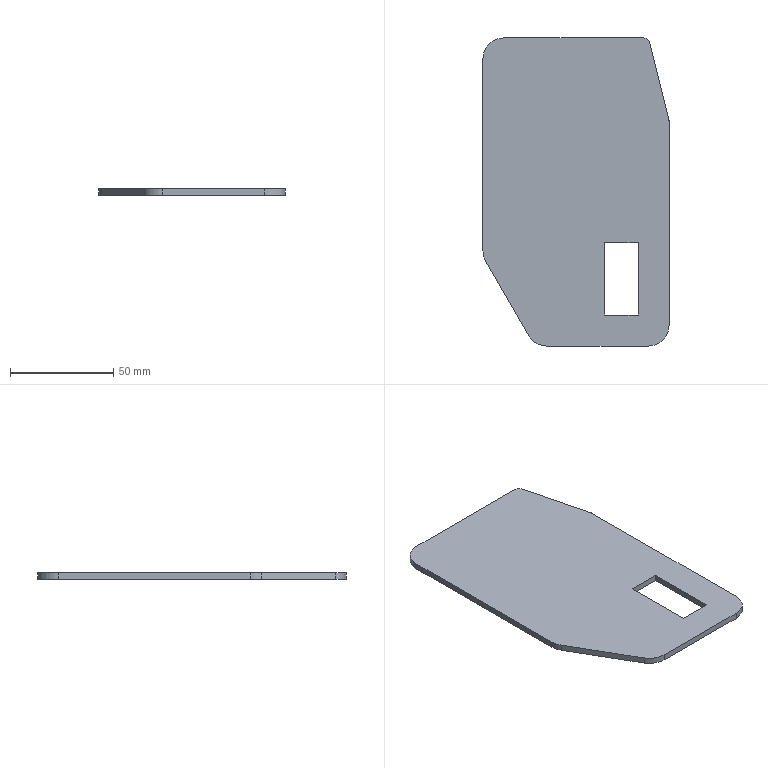Part | STEP file | Q7C1202R | 1 solid | 18 faces | box 90 x 149 x 3 mm | volume 36176 mm3 | plane 12 | cylinder 6 | commonest cylinder face diameters 20 x4 6 x2
STEP:
#1=CARTESIAN_POINT('',(0.,0.,0.));
#2=DIRECTION('',(0.,0.,1.));
#3=DIRECTION('',(1.,0.,0.));
#4=AXIS2_PLACEMENT_3D('',#1,#2,#3);
#5=CARTESIAN_POINT('',(45.,-64.5,-1.5));
#6=VERTEX_POINT('',#5);
#7=CARTESIAN_POINT('',(45.,34.131,-1.5));
#8=VERTEX_POINT('',#7);
#9=CARTESIAN_POINT('',(45.,-74.5,-1.5));
#10=DIRECTION('',(0.,1.,0.));
#11=VECTOR('',#10,1.);
#12=LINE('',#9,#11);
#13=CARTESIAN_POINT('',(45.,-74.5,1.5));
#14=DIRECTION('',(-1.,0.,0.));
#15=DIRECTION('',(0.,0.,1.));
#16=AXIS2_PLACEMENT_3D('',#13,#14,#15);
#17=PLANE('',#16);
#18=CARTESIAN_POINT('',(-3.,0.));
#19=DIRECTION('',(0.,1.));
#20=VECTOR('',#19,1.);
#21=LINE('',#18,#20);
#22=(GEOMETRIC_REPRESENTATION_CONTEXT(2)PARAMETRIC_REPRESENTATION_CONTEXT()REPRESENTATION_CONTEXT('',''));
#23=DEFINITIONAL_REPRESENTATION('',(#21),#22);
#24=PCURVE('',#17,#23);
#25=CARTESIAN_POINT('',(45.,74.5,-1.5));
#26=DIRECTION('',(0.,0.,1.));
#27=DIRECTION('',(1.,0.,0.));
#28=AXIS2_PLACEMENT_3D('',#25,#26,#27);
#29=PLANE('',#28);
#30=CARTESIAN_POINT('',(0.,-149.));
#31=DIRECTION('',(0.,1.));
#32=VECTOR('',#31,1.);
#33=LINE('',#30,#32);
#34=(GEOMETRIC_REPRESENTATION_CONTEXT(2)PARAMETRIC_REPRESENTATION_CONTEXT()REPRESENTATION_CONTEXT('',''));
#35=DEFINITIONAL_REPRESENTATION('',(#33),#34);
#36=PCURVE('',#29,#35);
#37=SURFACE_CURVE('',#12,(#24,#36),.PCURVE_S1.);
#38=EDGE_CURVE('',#6,#8,#37,.T.);
#39=ORIENTED_EDGE('',*,*,#38,.T.);
#40=CARTESIAN_POINT('',(45.,34.131,1.5));
#41=VERTEX_POINT('',#40);
#42=CARTESIAN_POINT('',(45.,34.131,1.5));
#43=DIRECTION('',(0.,0.,1.));
#44=VECTOR('',#43,1.);
#45=LINE('',#42,#44);
#46=CARTESIAN_POINT('',(0.,108.631));
#47=DIRECTION('',(1.,0.));
#48=VECTOR('',#47,1.);
#49=LINE('',#46,#48);
#50=(GEOMETRIC_REPRESENTATION_CONTEXT(2)PARAMETRIC_REPRESENTATION_CONTEXT()REPRESENTATION_CONTEXT('',''));
#51=DEFINITIONAL_REPRESENTATION('',(#49),#50);
#52=PCURVE('',#17,#51);
#53=CARTESIAN_POINT('',(42.,34.131,1.5));
#54=DIRECTION('',(0.,0.,1.));
#55=DIRECTION('',(1.,0.,0.));
#56=AXIS2_PLACEMENT_3D('',#53,#54,#55);
#57=CYLINDRICAL_SURFACE('',#56,3.);
#58=CARTESIAN_POINT('',(0.,0.));
#59=DIRECTION('',(0.,1.));
#60=VECTOR('',#59,1.);
#61=LINE('',#58,#60);
#62=(GEOMETRIC_REPRESENTATION_CONTEXT(2)PARAMETRIC_REPRESENTATION_CONTEXT()REPRESENTATION_CONTEXT('',''));
#63=DEFINITIONAL_REPRESENTATION('',(#61),#62);
#64=PCURVE('',#57,#63);
#65=SURFACE_CURVE('',#45,(#52,#64),.PCURVE_S1.);
#66=EDGE_CURVE('',#8,#41,#65,.T.);
#67=ORIENTED_EDGE('',*,*,#66,.T.);
#68=CARTESIAN_POINT('',(45.,-64.5,1.5));
#69=VERTEX_POINT('',#68);
#70=CARTESIAN_POINT('',(45.,-74.5,1.5));
#71=DIRECTION('',(0.,1.,0.));
#72=VECTOR('',#71,1.);
#73=LINE('',#70,#72);
#74=CARTESIAN_POINT('',(0.,0.));
#75=DIRECTION('',(0.,1.));
#76=VECTOR('',#75,1.);
#77=LINE('',#74,#76);
#78=(GEOMETRIC_REPRESENTATION_CONTEXT(2)PARAMETRIC_REPRESENTATION_CONTEXT()REPRESENTATION_CONTEXT('',''));
#79=DEFINITIONAL_REPRESENTATION('',(#77),#78);
#80=PCURVE('',#17,#79);
#81=CARTESIAN_POINT('',(45.,74.5,1.5));
#82=DIRECTION('',(0.,0.,1.));
#83=DIRECTION('',(1.,0.,0.));
#84=AXIS2_PLACEMENT_3D('',#81,#82,#83);
#85=PLANE('',#84);
#86=CARTESIAN_POINT('',(0.,-149.));
#87=DIRECTION('',(0.,1.));
#88=VECTOR('',#87,1.);
#89=LINE('',#86,#88);
#90=(GEOMETRIC_REPRESENTATION_CONTEXT(2)PARAMETRIC_REPRESENTATION_CONTEXT()REPRESENTATION_CONTEXT('',''));
#91=DEFINITIONAL_REPRESENTATION('',(#89),#90);
#92=PCURVE('',#85,#91);
#93=SURFACE_CURVE('',#73,(#80,#92),.PCURVE_S1.);
#94=EDGE_CURVE('',#69,#41,#93,.T.);
#95=ORIENTED_EDGE('',*,*,#94,.F.);
#96=CARTESIAN_POINT('',(45.,-64.5,1.5));
#97=DIRECTION('',(0.,0.,-1.));
#98=VECTOR('',#97,1.);
#99=LINE('',#96,#98);
#100=CARTESIAN_POINT('',(0.,10.));
#101=DIRECTION('',(-1.,0.));
#102=VECTOR('',#101,1.);
#103=LINE('',#100,#102);
#104=(GEOMETRIC_REPRESENTATION_CONTEXT(2)PARAMETRIC_REPRESENTATION_CONTEXT()REPRESENTATION_CONTEXT('',''));
#105=DEFINITIONAL_REPRESENTATION('',(#103),#104);
#106=PCURVE('',#17,#105);
#107=CARTESIAN_POINT('',(35.,-64.5,1.5));
#108=DIRECTION('',(0.,0.,-1.));
#109=DIRECTION('',(-1.,0.,0.));
#110=AXIS2_PLACEMENT_3D('',#107,#108,#109);
#111=CYLINDRICAL_SURFACE('',#110,10.);
#112=CARTESIAN_POINT('',(3.142,0.));
#113=DIRECTION('',(0.,1.));
#114=VECTOR('',#113,1.);
#115=LINE('',#112,#114);
#116=(GEOMETRIC_REPRESENTATION_CONTEXT(2)PARAMETRIC_REPRESENTATION_CONTEXT()REPRESENTATION_CONTEXT('',''));
#117=DEFINITIONAL_REPRESENTATION('',(#115),#116);
#118=PCURVE('',#111,#117);
#119=SURFACE_CURVE('',#99,(#106,#118),.PCURVE_S1.);
#120=EDGE_CURVE('',#69,#6,#119,.T.);
#121=ORIENTED_EDGE('',*,*,#120,.T.);
#122=EDGE_LOOP('',(#39,#67,#95,#121));
#123=FACE_BOUND('',#122,.T.);
#124=ADVANCED_FACE('',(#123),#17,.F.);
#125=CARTESIAN_POINT('',(32.658,74.5,1.5));
#126=VERTEX_POINT('',#125);
#127=CARTESIAN_POINT('',(-35.,74.5,1.5));
#128=VERTEX_POINT('',#127);
#129=CARTESIAN_POINT('',(45.,74.5,1.5));
#130=DIRECTION('',(-1.,0.,0.));
#131=VECTOR('',#130,1.);
#132=LINE('',#129,#131);
#133=CARTESIAN_POINT('',(45.,74.5,1.5));
#134=DIRECTION('',(0.,-1.,0.));
#135=DIRECTION('',(0.,0.,-1.));
#136=AXIS2_PLACEMENT_3D('',#133,#134,#135);
#137=PLANE('',#136);
#138=CARTESIAN_POINT('',(0.,0.));
#139=DIRECTION('',(0.,-1.));
#140=VECTOR('',#139,1.);
#141=LINE('',#138,#140);
#142=(GEOMETRIC_REPRESENTATION_CONTEXT(2)PARAMETRIC_REPRESENTATION_CONTEXT()REPRESENTATION_CONTEXT('',''));
#143=DEFINITIONAL_REPRESENTATION('',(#141),#142);
#144=PCURVE('',#137,#143);
#145=CARTESIAN_POINT('',(0.,0.));
#146=DIRECTION('',(-1.,0.));
#147=VECTOR('',#146,1.);
#148=LINE('',#145,#147);
#149=(GEOMETRIC_REPRESENTATION_CONTEXT(2)PARAMETRIC_REPRESENTATION_CONTEXT()REPRESENTATION_CONTEXT('',''));
#150=DEFINITIONAL_REPRESENTATION('',(#148),#149);
#151=PCURVE('',#85,#150);
#152=SURFACE_CURVE('',#132,(#144,#151),.PCURVE_S1.);
#153=EDGE_CURVE('',#126,#128,#152,.T.);
#154=ORIENTED_EDGE('',*,*,#153,.F.);
#155=CARTESIAN_POINT('',(32.658,74.5,-1.5));
#156=VERTEX_POINT('',#155);
#157=CARTESIAN_POINT('',(32.658,74.5,1.5));
#158=DIRECTION('',(0.,0.,-1.));
#159=VECTOR('',#158,1.);
#160=LINE('',#157,#159);
#161=CARTESIAN_POINT('',(0.,-12.342));
#162=DIRECTION('',(1.,0.));
#163=VECTOR('',#162,1.);
#164=LINE('',#161,#163);
#165=(GEOMETRIC_REPRESENTATION_CONTEXT(2)PARAMETRIC_REPRESENTATION_CONTEXT()REPRESENTATION_CONTEXT('',''));
#166=DEFINITIONAL_REPRESENTATION('',(#164),#165);
#167=PCURVE('',#137,#166);
#168=CARTESIAN_POINT('',(32.658,71.5,1.5));
#169=DIRECTION('',(0.,0.,-1.));
#170=DIRECTION('',(-1.,0.,0.));
#171=AXIS2_PLACEMENT_3D('',#168,#169,#170);
#172=CYLINDRICAL_SURFACE('',#171,3.);
#173=CARTESIAN_POINT('',(1.571,0.));
#174=DIRECTION('',(0.,1.));
#175=VECTOR('',#174,1.);
#176=LINE('',#173,#175);
#177=(GEOMETRIC_REPRESENTATION_CONTEXT(2)PARAMETRIC_REPRESENTATION_CONTEXT()REPRESENTATION_CONTEXT('',''));
#178=DEFINITIONAL_REPRESENTATION('',(#176),#177);
#179=PCURVE('',#172,#178);
#180=SURFACE_CURVE('',#160,(#167,#179),.PCURVE_S1.);
#181=EDGE_CURVE('',#126,#156,#180,.T.);
#182=ORIENTED_EDGE('',*,*,#181,.T.);
#183=CARTESIAN_POINT('',(-35.,74.5,-1.5));
#184=VERTEX_POINT('',#183);
#185=CARTESIAN_POINT('',(45.,74.5,-1.5));
#186=DIRECTION('',(-1.,0.,0.));
#187=VECTOR('',#186,1.);
#188=LINE('',#185,#187);
#189=CARTESIAN_POINT('',(3.,0.));
#190=DIRECTION('',(0.,-1.));
#191=VECTOR('',#190,1.);
#192=LINE('',#189,#191);
#193=(GEOMETRIC_REPRESENTATION_CONTEXT(2)PARAMETRIC_REPRESENTATION_CONTEXT()REPRESENTATION_CONTEXT('',''));
#194=DEFINITIONAL_REPRESENTATION('',(#192),#193);
#195=PCURVE('',#137,#194);
#196=CARTESIAN_POINT('',(0.,0.));
#197=DIRECTION('',(-1.,0.));
#198=VECTOR('',#197,1.);
#199=LINE('',#196,#198);
#200=(GEOMETRIC_REPRESENTATION_CONTEXT(2)PARAMETRIC_REPRESENTATION_CONTEXT()REPRESENTATION_CONTEXT('',''));
#201=DEFINITIONAL_REPRESENTATION('',(#199),#200);
#202=PCURVE('',#29,#201);
#203=SURFACE_CURVE('',#188,(#195,#202),.PCURVE_S1.);
#204=EDGE_CURVE('',#156,#184,#203,.T.);
#205=ORIENTED_EDGE('',*,*,#204,.T.);
#206=CARTESIAN_POINT('',(-35.,74.5,1.5));
#207=DIRECTION('',(0.,0.,1.));
#208=VECTOR('',#207,1.);
#209=LINE('',#206,#208);
#210=CARTESIAN_POINT('',(0.,-80.));
#211=DIRECTION('',(-1.,0.));
#212=VECTOR('',#211,1.);
#213=LINE('',#210,#212);
#214=(GEOMETRIC_REPRESENTATION_CONTEXT(2)PARAMETRIC_REPRESENTATION_CONTEXT()REPRESENTATION_CONTEXT('',''));
#215=DEFINITIONAL_REPRESENTATION('',(#213),#214);
#216=PCURVE('',#137,#215);
#217=CARTESIAN_POINT('',(-35.,64.5,1.5));
#218=DIRECTION('',(0.,0.,-1.));
#219=DIRECTION('',(-1.,0.,0.));
#220=AXIS2_PLACEMENT_3D('',#217,#218,#219);
#221=CYLINDRICAL_SURFACE('',#220,10.);
#222=CARTESIAN_POINT('',(1.571,0.));
#223=DIRECTION('',(0.,-1.));
#224=VECTOR('',#223,1.);
#225=LINE('',#222,#224);
#226=(GEOMETRIC_REPRESENTATION_CONTEXT(2)PARAMETRIC_REPRESENTATION_CONTEXT()REPRESENTATION_CONTEXT('',''));
#227=DEFINITIONAL_REPRESENTATION('',(#225),#226);
#228=PCURVE('',#221,#227);
#229=SURFACE_CURVE('',#209,(#216,#228),.PCURVE_S1.);
#230=EDGE_CURVE('',#184,#128,#229,.T.);
#231=ORIENTED_EDGE('',*,*,#230,.T.);
#232=EDGE_LOOP('',(#154,#182,#205,#231));
#233=FACE_BOUND('',#232,.T.);
#234=ADVANCED_FACE('',(#233),#137,.F.);
#235=CARTESIAN_POINT('',(-45.,64.5,-1.5));
#236=VERTEX_POINT('',#235);
#237=CARTESIAN_POINT('',(-45.,-28.519,-1.5));
#238=VERTEX_POINT('',#237);
#239=CARTESIAN_POINT('',(-45.,74.5,-1.5));
#240=DIRECTION('',(0.,-1.,0.));
#241=VECTOR('',#240,1.);
#242=LINE('',#239,#241);
#243=CARTESIAN_POINT('',(-45.,74.5,1.5));
#244=DIRECTION('',(1.,0.,0.));
#245=DIRECTION('',(0.,1.,0.));
#246=AXIS2_PLACEMENT_3D('',#243,#244,#245);
#247=PLANE('',#246);
#248=CARTESIAN_POINT('',(0.,-3.));
#249=DIRECTION('',(-1.,0.));
#250=VECTOR('',#249,1.);
#251=LINE('',#248,#250);
#252=(GEOMETRIC_REPRESENTATION_CONTEXT(2)PARAMETRIC_REPRESENTATION_CONTEXT()REPRESENTATION_CONTEXT('',''));
#253=DEFINITIONAL_REPRESENTATION('',(#251),#252);
#254=PCURVE('',#247,#253);
#255=CARTESIAN_POINT('',(-90.,0.));
#256=DIRECTION('',(0.,-1.));
#257=VECTOR('',#256,1.);
#258=LINE('',#255,#257);
#259=(GEOMETRIC_REPRESENTATION_CONTEXT(2)PARAMETRIC_REPRESENTATION_CONTEXT()REPRESENTATION_CONTEXT('',''));
#260=DEFINITIONAL_REPRESENTATION('',(#258),#259);
#261=PCURVE('',#29,#260);
#262=SURFACE_CURVE('',#242,(#254,#261),.PCURVE_S1.);
#263=EDGE_CURVE('',#236,#238,#262,.T.);
#264=ORIENTED_EDGE('',*,*,#263,.T.);
#265=CARTESIAN_POINT('',(-45.,-28.519,1.5));
#266=VERTEX_POINT('',#265);
#267=CARTESIAN_POINT('',(-45.,-28.519,1.5));
#268=DIRECTION('',(0.,0.,1.));
#269=VECTOR('',#268,1.);
#270=LINE('',#267,#269);
#271=CARTESIAN_POINT('',(-103.019,0.));
#272=DIRECTION('',(0.,1.));
#273=VECTOR('',#272,1.);
#274=LINE('',#271,#273);
#275=(GEOMETRIC_REPRESENTATION_CONTEXT(2)PARAMETRIC_REPRESENTATION_CONTEXT()REPRESENTATION_CONTEXT('',''));
#276=DEFINITIONAL_REPRESENTATION('',(#274),#275);
#277=PCURVE('',#247,#276);
#278=CARTESIAN_POINT('',(-35.,-28.519,1.5));
#279=DIRECTION('',(0.,0.,-1.));
#280=DIRECTION('',(-1.,0.,0.));
#281=AXIS2_PLACEMENT_3D('',#278,#279,#280);
#282=CYLINDRICAL_SURFACE('',#281,10.);
#283=CARTESIAN_POINT('',(6.283,0.));
#284=DIRECTION('',(0.,-1.));
#285=VECTOR('',#284,1.);
#286=LINE('',#283,#285);
#287=(GEOMETRIC_REPRESENTATION_CONTEXT(2)PARAMETRIC_REPRESENTATION_CONTEXT()REPRESENTATION_CONTEXT('',''));
#288=DEFINITIONAL_REPRESENTATION('',(#286),#287);
#289=PCURVE('',#282,#288);
#290=SURFACE_CURVE('',#270,(#277,#289),.PCURVE_S1.);
#291=EDGE_CURVE('',#238,#266,#290,.T.);
#292=ORIENTED_EDGE('',*,*,#291,.T.);
#293=CARTESIAN_POINT('',(-45.,64.5,1.5));
#294=VERTEX_POINT('',#293);
#295=CARTESIAN_POINT('',(-45.,74.5,1.5));
#296=DIRECTION('',(0.,-1.,0.));
#297=VECTOR('',#296,1.);
#298=LINE('',#295,#297);
#299=CARTESIAN_POINT('',(0.,0.));
#300=DIRECTION('',(-1.,0.));
#301=VECTOR('',#300,1.);
#302=LINE('',#299,#301);
#303=(GEOMETRIC_REPRESENTATION_CONTEXT(2)PARAMETRIC_REPRESENTATION_CONTEXT()REPRESENTATION_CONTEXT('',''));
#304=DEFINITIONAL_REPRESENTATION('',(#302),#303);
#305=PCURVE('',#247,#304);
#306=CARTESIAN_POINT('',(-90.,0.));
#307=DIRECTION('',(0.,-1.));
#308=VECTOR('',#307,1.);
#309=LINE('',#306,#308);
#310=(GEOMETRIC_REPRESENTATION_CONTEXT(2)PARAMETRIC_REPRESENTATION_CONTEXT()REPRESENTATION_CONTEXT('',''));
#311=DEFINITIONAL_REPRESENTATION('',(#309),#310);
#312=PCURVE('',#85,#311);
#313=SURFACE_CURVE('',#298,(#305,#312),.PCURVE_S1.);
#314=EDGE_CURVE('',#294,#266,#313,.T.);
#315=ORIENTED_EDGE('',*,*,#314,.F.);
#316=CARTESIAN_POINT('',(-45.,64.5,1.5));
#317=DIRECTION('',(0.,0.,-1.));
#318=VECTOR('',#317,1.);
#319=LINE('',#316,#318);
#320=CARTESIAN_POINT('',(-10.,0.));
#321=DIRECTION('',(0.,-1.));
#322=VECTOR('',#321,1.);
#323=LINE('',#320,#322);
#324=(GEOMETRIC_REPRESENTATION_CONTEXT(2)PARAMETRIC_REPRESENTATION_CONTEXT()REPRESENTATION_CONTEXT('',''));
#325=DEFINITIONAL_REPRESENTATION('',(#323),#324);
#326=PCURVE('',#247,#325);
#327=CARTESIAN_POINT('',(0.,0.));
#328=DIRECTION('',(0.,1.));
#329=VECTOR('',#328,1.);
#330=LINE('',#327,#329);
#331=(GEOMETRIC_REPRESENTATION_CONTEXT(2)PARAMETRIC_REPRESENTATION_CONTEXT()REPRESENTATION_CONTEXT('',''));
#332=DEFINITIONAL_REPRESENTATION('',(#330),#331);
#333=PCURVE('',#221,#332);
#334=SURFACE_CURVE('',#319,(#326,#333),.PCURVE_S1.);
#335=EDGE_CURVE('',#294,#236,#334,.T.);
#336=ORIENTED_EDGE('',*,*,#335,.T.);
#337=EDGE_LOOP('',(#264,#292,#315,#336));
#338=FACE_BOUND('',#337,.T.);
#339=ADVANCED_FACE('',(#338),#247,.F.);
#340=CARTESIAN_POINT('',(-43.66,-33.519,1.5));
#341=VERTEX_POINT('',#340);
#342=CARTESIAN_POINT('',(-22.887,-69.5,1.5));
#343=VERTEX_POINT('',#342);
#344=CARTESIAN_POINT('',(-45.,-31.199,1.5));
#345=DIRECTION('',(0.5,-0.866,0.));
#346=VECTOR('',#345,1.);
#347=LINE('',#344,#346);
#348=CARTESIAN_POINT('',(-45.,-31.199,1.5));
#349=DIRECTION('',(0.866,0.5,0.));
#350=DIRECTION('',(-0.5,0.866,0.));
#351=AXIS2_PLACEMENT_3D('',#348,#349,#350);
#352=PLANE('',#351);
#353=CARTESIAN_POINT('',(0.,0.));
#354=DIRECTION('',(-1.,0.));
#355=VECTOR('',#354,1.);
#356=LINE('',#353,#355);
#357=(GEOMETRIC_REPRESENTATION_CONTEXT(2)PARAMETRIC_REPRESENTATION_CONTEXT()REPRESENTATION_CONTEXT('',''));
#358=DEFINITIONAL_REPRESENTATION('',(#356),#357);
#359=PCURVE('',#352,#358);
#360=CARTESIAN_POINT('',(-90.,-105.699));
#361=DIRECTION('',(0.5,-0.866));
#362=VECTOR('',#361,1.);
#363=LINE('',#360,#362);
#364=(GEOMETRIC_REPRESENTATION_CONTEXT(2)PARAMETRIC_REPRESENTATION_CONTEXT()REPRESENTATION_CONTEXT('',''));
#365=DEFINITIONAL_REPRESENTATION('',(#363),#364);
#366=PCURVE('',#85,#365);
#367=SURFACE_CURVE('',#347,(#359,#366),.PCURVE_S1.);
#368=EDGE_CURVE('',#341,#343,#367,.T.);
#369=ORIENTED_EDGE('',*,*,#368,.F.);
#370=CARTESIAN_POINT('',(-43.66,-33.519,-1.5));
#371=VERTEX_POINT('',#370);
#372=CARTESIAN_POINT('',(-43.66,-33.519,1.5));
#373=DIRECTION('',(0.,0.,-1.));
#374=VECTOR('',#373,1.);
#375=LINE('',#372,#374);
#376=CARTESIAN_POINT('',(-2.679,0.));
#377=DIRECTION('',(0.,-1.));
#378=VECTOR('',#377,1.);
#379=LINE('',#376,#378);
#380=(GEOMETRIC_REPRESENTATION_CONTEXT(2)PARAMETRIC_REPRESENTATION_CONTEXT()REPRESENTATION_CONTEXT('',''));
#381=DEFINITIONAL_REPRESENTATION('',(#379),#380);
#382=PCURVE('',#352,#381);
#383=CARTESIAN_POINT('',(5.76,0.));
#384=DIRECTION('',(0.,1.));
#385=VECTOR('',#384,1.);
#386=LINE('',#383,#385);
#387=(GEOMETRIC_REPRESENTATION_CONTEXT(2)PARAMETRIC_REPRESENTATION_CONTEXT()REPRESENTATION_CONTEXT('',''));
#388=DEFINITIONAL_REPRESENTATION('',(#386),#387);
#389=PCURVE('',#282,#388);
#390=SURFACE_CURVE('',#375,(#382,#389),.PCURVE_S1.);
#391=EDGE_CURVE('',#341,#371,#390,.T.);
#392=ORIENTED_EDGE('',*,*,#391,.T.);
#393=CARTESIAN_POINT('',(-22.887,-69.5,-1.5));
#394=VERTEX_POINT('',#393);
#395=CARTESIAN_POINT('',(-45.,-31.199,-1.5));
#396=DIRECTION('',(0.5,-0.866,0.));
#397=VECTOR('',#396,1.);
#398=LINE('',#395,#397);
#399=CARTESIAN_POINT('',(0.,-3.));
#400=DIRECTION('',(-1.,0.));
#401=VECTOR('',#400,1.);
#402=LINE('',#399,#401);
#403=(GEOMETRIC_REPRESENTATION_CONTEXT(2)PARAMETRIC_REPRESENTATION_CONTEXT()REPRESENTATION_CONTEXT('',''));
#404=DEFINITIONAL_REPRESENTATION('',(#402),#403);
#405=PCURVE('',#352,#404);
#406=CARTESIAN_POINT('',(-90.,-105.699));
#407=DIRECTION('',(0.5,-0.866));
#408=VECTOR('',#407,1.);
#409=LINE('',#406,#408);
#410=(GEOMETRIC_REPRESENTATION_CONTEXT(2)PARAMETRIC_REPRESENTATION_CONTEXT()REPRESENTATION_CONTEXT('',''));
#411=DEFINITIONAL_REPRESENTATION('',(#409),#410);
#412=PCURVE('',#29,#411);
#413=SURFACE_CURVE('',#398,(#405,#412),.PCURVE_S1.);
#414=EDGE_CURVE('',#371,#394,#413,.T.);
#415=ORIENTED_EDGE('',*,*,#414,.T.);
#416=CARTESIAN_POINT('',(-22.887,-69.5,1.5));
#417=DIRECTION('',(0.,0.,1.));
#418=VECTOR('',#417,1.);
#419=LINE('',#416,#418);
#420=CARTESIAN_POINT('',(-44.226,0.));
#421=DIRECTION('',(0.,1.));
#422=VECTOR('',#421,1.);
#423=LINE('',#420,#422);
#424=(GEOMETRIC_REPRESENTATION_CONTEXT(2)PARAMETRIC_REPRESENTATION_CONTEXT()REPRESENTATION_CONTEXT('',''));
#425=DEFINITIONAL_REPRESENTATION('',(#423),#424);
#426=PCURVE('',#352,#425);
#427=CARTESIAN_POINT('',(-14.226,-64.5,1.5));
#428=DIRECTION('',(0.,0.,-1.));
#429=DIRECTION('',(-1.,0.,0.));
#430=AXIS2_PLACEMENT_3D('',#427,#428,#429);
#431=CYLINDRICAL_SURFACE('',#430,10.);
#432=CARTESIAN_POINT('',(5.76,0.));
#433=DIRECTION('',(0.,-1.));
#434=VECTOR('',#433,1.);
#435=LINE('',#432,#434);
#436=(GEOMETRIC_REPRESENTATION_CONTEXT(2)PARAMETRIC_REPRESENTATION_CONTEXT()REPRESENTATION_CONTEXT('',''));
#437=DEFINITIONAL_REPRESENTATION('',(#435),#436);
#438=PCURVE('',#431,#437);
#439=SURFACE_CURVE('',#419,(#426,#438),.PCURVE_S1.);
#440=EDGE_CURVE('',#394,#343,#439,.T.);
#441=ORIENTED_EDGE('',*,*,#440,.T.);
#442=EDGE_LOOP('',(#369,#392,#415,#441));
#443=FACE_BOUND('',#442,.T.);
#444=ADVANCED_FACE('',(#443),#352,.F.);
#445=CARTESIAN_POINT('',(-14.226,-74.5,1.5));
#446=VERTEX_POINT('',#445);
#447=CARTESIAN_POINT('',(35.,-74.5,1.5));
#448=VERTEX_POINT('',#447);
#449=CARTESIAN_POINT('',(-20.,-74.5,1.5));
#450=DIRECTION('',(1.,0.,0.));
#451=VECTOR('',#450,1.);
#452=LINE('',#449,#451);
#453=CARTESIAN_POINT('',(-20.,-74.5,1.5));
#454=DIRECTION('',(0.,1.,0.));
#455=DIRECTION('',(0.,0.,1.));
#456=AXIS2_PLACEMENT_3D('',#453,#454,#455);
#457=PLANE('',#456);
#458=CARTESIAN_POINT('',(0.,0.));
#459=DIRECTION('',(0.,1.));
#460=VECTOR('',#459,1.);
#461=LINE('',#458,#460);
#462=(GEOMETRIC_REPRESENTATION_CONTEXT(2)PARAMETRIC_REPRESENTATION_CONTEXT()REPRESENTATION_CONTEXT('',''));
#463=DEFINITIONAL_REPRESENTATION('',(#461),#462);
#464=PCURVE('',#457,#463);
#465=CARTESIAN_POINT('',(-65.,-149.));
#466=DIRECTION('',(1.,0.));
#467=VECTOR('',#466,1.);
#468=LINE('',#465,#467);
#469=(GEOMETRIC_REPRESENTATION_CONTEXT(2)PARAMETRIC_REPRESENTATION_CONTEXT()REPRESENTATION_CONTEXT('',''));
#470=DEFINITIONAL_REPRESENTATION('',(#468),#469);
#471=PCURVE('',#85,#470);
#472=SURFACE_CURVE('',#452,(#464,#471),.PCURVE_S1.);
#473=EDGE_CURVE('',#446,#448,#472,.T.);
#474=ORIENTED_EDGE('',*,*,#473,.F.);
#475=CARTESIAN_POINT('',(-14.226,-74.5,-1.5));
#476=VERTEX_POINT('',#475);
#477=CARTESIAN_POINT('',(-14.226,-74.5,1.5));
#478=DIRECTION('',(0.,0.,-1.));
#479=VECTOR('',#478,1.);
#480=LINE('',#477,#479);
#481=CARTESIAN_POINT('',(0.,5.774));
#482=DIRECTION('',(-1.,0.));
#483=VECTOR('',#482,1.);
#484=LINE('',#481,#483);
#485=(GEOMETRIC_REPRESENTATION_CONTEXT(2)PARAMETRIC_REPRESENTATION_CONTEXT()REPRESENTATION_CONTEXT('',''));
#486=DEFINITIONAL_REPRESENTATION('',(#484),#485);
#487=PCURVE('',#457,#486);
#488=CARTESIAN_POINT('',(4.712,0.));
#489=DIRECTION('',(0.,1.));
#490=VECTOR('',#489,1.);
#491=LINE('',#488,#490);
#492=(GEOMETRIC_REPRESENTATION_CONTEXT(2)PARAMETRIC_REPRESENTATION_CONTEXT()REPRESENTATION_CONTEXT('',''));
#493=DEFINITIONAL_REPRESENTATION('',(#491),#492);
#494=PCURVE('',#431,#493);
#495=SURFACE_CURVE('',#480,(#487,#494),.PCURVE_S1.);
#496=EDGE_CURVE('',#446,#476,#495,.T.);
#497=ORIENTED_EDGE('',*,*,#496,.T.);
#498=CARTESIAN_POINT('',(35.,-74.5,-1.5));
#499=VERTEX_POINT('',#498);
#500=CARTESIAN_POINT('',(-20.,-74.5,-1.5));
#501=DIRECTION('',(1.,0.,0.));
#502=VECTOR('',#501,1.);
#503=LINE('',#500,#502);
#504=CARTESIAN_POINT('',(-3.,0.));
#505=DIRECTION('',(0.,1.));
#506=VECTOR('',#505,1.);
#507=LINE('',#504,#506);
#508=(GEOMETRIC_REPRESENTATION_CONTEXT(2)PARAMETRIC_REPRESENTATION_CONTEXT()REPRESENTATION_CONTEXT('',''));
#509=DEFINITIONAL_REPRESENTATION('',(#507),#508);
#510=PCURVE('',#457,#509);
#511=CARTESIAN_POINT('',(-65.,-149.));
#512=DIRECTION('',(1.,0.));
#513=VECTOR('',#512,1.);
#514=LINE('',#511,#513);
#515=(GEOMETRIC_REPRESENTATION_CONTEXT(2)PARAMETRIC_REPRESENTATION_CONTEXT()REPRESENTATION_CONTEXT('',''));
#516=DEFINITIONAL_REPRESENTATION('',(#514),#515);
#517=PCURVE('',#29,#516);
#518=SURFACE_CURVE('',#503,(#510,#517),.PCURVE_S1.);
#519=EDGE_CURVE('',#476,#499,#518,.T.);
#520=ORIENTED_EDGE('',*,*,#519,.T.);
#521=CARTESIAN_POINT('',(35.,-74.5,1.5));
#522=DIRECTION('',(0.,0.,1.));
#523=VECTOR('',#522,1.);
#524=LINE('',#521,#523);
#525=CARTESIAN_POINT('',(0.,55.));
#526=DIRECTION('',(1.,0.));
#527=VECTOR('',#526,1.);
#528=LINE('',#525,#527);
#529=(GEOMETRIC_REPRESENTATION_CONTEXT(2)PARAMETRIC_REPRESENTATION_CONTEXT()REPRESENTATION_CONTEXT('',''));
#530=DEFINITIONAL_REPRESENTATION('',(#528),#529);
#531=PCURVE('',#457,#530);
#532=CARTESIAN_POINT('',(4.712,0.));
#533=DIRECTION('',(0.,-1.));
#534=VECTOR('',#533,1.);
#535=LINE('',#532,#534);
#536=(GEOMETRIC_REPRESENTATION_CONTEXT(2)PARAMETRIC_REPRESENTATION_CONTEXT()REPRESENTATION_CONTEXT('',''));
#537=DEFINITIONAL_REPRESENTATION('',(#535),#536);
#538=PCURVE('',#111,#537);
#539=SURFACE_CURVE('',#524,(#531,#538),.PCURVE_S1.);
#540=EDGE_CURVE('',#499,#448,#539,.T.);
#541=ORIENTED_EDGE('',*,*,#540,.T.);
#542=EDGE_LOOP('',(#474,#497,#520,#541));
#543=FACE_BOUND('',#542,.T.);
#544=ADVANCED_FACE('',(#543),#457,.F.);
#545=ORIENTED_EDGE('',*,*,#94,.T.);
#546=CARTESIAN_POINT('',(44.91,34.858,1.5));
#547=VERTEX_POINT('',#546);
#548=CARTESIAN_POINT('',(42.,34.131,1.5));
#549=DIRECTION('',(0.,0.,1.));
#550=DIRECTION('',(1.,0.,0.));
#551=AXIS2_PLACEMENT_3D('',#548,#549,#550);
#552=CIRCLE('',#551,3.);
#553=CARTESIAN_POINT('',(-3.,-40.369));
#554=DIRECTION('',(1.,0.));
#555=AXIS2_PLACEMENT_2D('',#553,#554);
#556=CIRCLE('',#555,3.);
#557=(GEOMETRIC_REPRESENTATION_CONTEXT(2)PARAMETRIC_REPRESENTATION_CONTEXT()REPRESENTATION_CONTEXT('',''));
#558=DEFINITIONAL_REPRESENTATION('',(#556),#557);
#559=PCURVE('',#85,#558);
#560=CARTESIAN_POINT('',(0.,0.));
#561=DIRECTION('',(1.,0.));
#562=VECTOR('',#561,1.);
#563=LINE('',#560,#562);
#564=(GEOMETRIC_REPRESENTATION_CONTEXT(2)PARAMETRIC_REPRESENTATION_CONTEXT()REPRESENTATION_CONTEXT('',''));
#565=DEFINITIONAL_REPRESENTATION('',(#563),#564);
#566=PCURVE('',#57,#565);
#567=SURFACE_CURVE('',#552,(#559,#566),.PCURVE_S1.);
#568=EDGE_CURVE('',#41,#547,#567,.T.);
#569=ORIENTED_EDGE('',*,*,#568,.T.);
#570=CARTESIAN_POINT('',(35.568,72.228,1.5));
#571=VERTEX_POINT('',#570);
#572=CARTESIAN_POINT('',(35.,74.5,1.5));
#573=DIRECTION('',(0.2425,-0.9701,0.));
#574=VECTOR('',#573,1.);
#575=LINE('',#572,#574);
#576=CARTESIAN_POINT('',(-10.,0.));
#577=DIRECTION('',(0.2425,-0.9701));
#578=VECTOR('',#577,1.);
#579=LINE('',#576,#578);
#580=(GEOMETRIC_REPRESENTATION_CONTEXT(2)PARAMETRIC_REPRESENTATION_CONTEXT()REPRESENTATION_CONTEXT('',''));
#581=DEFINITIONAL_REPRESENTATION('',(#579),#580);
#582=PCURVE('',#85,#581);
#583=CARTESIAN_POINT('',(35.,74.5,-8.5));
#584=DIRECTION('',(-0.9701,-0.2425,0.));
#585=DIRECTION('',(0.2425,-0.9701,0.));
#586=AXIS2_PLACEMENT_3D('',#583,#584,#585);
#587=PLANE('',#586);
#588=CARTESIAN_POINT('',(0.,10.));
#589=DIRECTION('',(1.,0.));
#590=VECTOR('',#589,1.);
#591=LINE('',#588,#590);
#592=(GEOMETRIC_REPRESENTATION_CONTEXT(2)PARAMETRIC_REPRESENTATION_CONTEXT()REPRESENTATION_CONTEXT('',''));
#593=DEFINITIONAL_REPRESENTATION('',(#591),#592);
#594=PCURVE('',#587,#593);
#595=SURFACE_CURVE('',#575,(#582,#594),.PCURVE_S1.);
#596=EDGE_CURVE('',#571,#547,#595,.T.);
#597=ORIENTED_EDGE('',*,*,#596,.F.);
#598=CARTESIAN_POINT('',(32.658,71.5,1.5));
#599=DIRECTION('',(0.,0.,1.));
#600=DIRECTION('',(1.,0.,0.));
#601=AXIS2_PLACEMENT_3D('',#598,#599,#600);
#602=CIRCLE('',#601,3.);
#603=CARTESIAN_POINT('',(-12.342,-3.));
#604=DIRECTION('',(1.,0.));
#605=AXIS2_PLACEMENT_2D('',#603,#604);
#606=CIRCLE('',#605,3.);
#607=(GEOMETRIC_REPRESENTATION_CONTEXT(2)PARAMETRIC_REPRESENTATION_CONTEXT()REPRESENTATION_CONTEXT('',''));
#608=DEFINITIONAL_REPRESENTATION('',(#606),#607);
#609=PCURVE('',#85,#608);
#610=CARTESIAN_POINT('',(3.142,0.));
#611=DIRECTION('',(-1.,0.));
#612=VECTOR('',#611,1.);
#613=LINE('',#610,#612);
#614=(GEOMETRIC_REPRESENTATION_CONTEXT(2)PARAMETRIC_REPRESENTATION_CONTEXT()REPRESENTATION_CONTEXT('',''));
#615=DEFINITIONAL_REPRESENTATION('',(#613),#614);
#616=PCURVE('',#172,#615);
#617=SURFACE_CURVE('',#602,(#609,#616),.PCURVE_S1.);
#618=EDGE_CURVE('',#571,#126,#617,.T.);
#619=ORIENTED_EDGE('',*,*,#618,.T.);
#620=ORIENTED_EDGE('',*,*,#153,.T.);
#621=CARTESIAN_POINT('',(-35.,64.5,1.5));
#622=DIRECTION('',(0.,0.,1.));
#623=DIRECTION('',(1.,0.,0.));
#624=AXIS2_PLACEMENT_3D('',#621,#622,#623);
#625=CIRCLE('',#624,10.);
#626=CARTESIAN_POINT('',(-80.,-10.));
#627=DIRECTION('',(1.,0.));
#628=AXIS2_PLACEMENT_2D('',#626,#627);
#629=CIRCLE('',#628,10.);
#630=(GEOMETRIC_REPRESENTATION_CONTEXT(2)PARAMETRIC_REPRESENTATION_CONTEXT()REPRESENTATION_CONTEXT('',''));
#631=DEFINITIONAL_REPRESENTATION('',(#629),#630);
#632=PCURVE('',#85,#631);
#633=CARTESIAN_POINT('',(3.142,0.));
#634=DIRECTION('',(-1.,0.));
#635=VECTOR('',#634,1.);
#636=LINE('',#633,#635);
#637=(GEOMETRIC_REPRESENTATION_CONTEXT(2)PARAMETRIC_REPRESENTATION_CONTEXT()REPRESENTATION_CONTEXT('',''));
#638=DEFINITIONAL_REPRESENTATION('',(#636),#637);
#639=PCURVE('',#221,#638);
#640=SURFACE_CURVE('',#625,(#632,#639),.PCURVE_S1.);
#641=EDGE_CURVE('',#128,#294,#640,.T.);
#642=ORIENTED_EDGE('',*,*,#641,.T.);
#643=ORIENTED_EDGE('',*,*,#314,.T.);
#644=CARTESIAN_POINT('',(-35.,-28.519,1.5));
#645=DIRECTION('',(0.,0.,1.));
#646=DIRECTION('',(1.,0.,0.));
#647=AXIS2_PLACEMENT_3D('',#644,#645,#646);
#648=CIRCLE('',#647,10.);
#649=CARTESIAN_POINT('',(-80.,-103.019));
#650=DIRECTION('',(1.,0.));
#651=AXIS2_PLACEMENT_2D('',#649,#650);
#652=CIRCLE('',#651,10.);
#653=(GEOMETRIC_REPRESENTATION_CONTEXT(2)PARAMETRIC_REPRESENTATION_CONTEXT()REPRESENTATION_CONTEXT('',''));
#654=DEFINITIONAL_REPRESENTATION('',(#652),#653);
#655=PCURVE('',#85,#654);
#656=CARTESIAN_POINT('',(9.425,0.));
#657=DIRECTION('',(-1.,0.));
#658=VECTOR('',#657,1.);
#659=LINE('',#656,#658);
#660=(GEOMETRIC_REPRESENTATION_CONTEXT(2)PARAMETRIC_REPRESENTATION_CONTEXT()REPRESENTATION_CONTEXT('',''));
#661=DEFINITIONAL_REPRESENTATION('',(#659),#660);
#662=PCURVE('',#282,#661);
#663=SURFACE_CURVE('',#648,(#655,#662),.PCURVE_S1.);
#664=EDGE_CURVE('',#266,#341,#663,.T.);
#665=ORIENTED_EDGE('',*,*,#664,.T.);
#666=ORIENTED_EDGE('',*,*,#368,.T.);
#667=CARTESIAN_POINT('',(-14.226,-64.5,1.5));
#668=DIRECTION('',(0.,0.,1.));
#669=DIRECTION('',(1.,0.,0.));
#670=AXIS2_PLACEMENT_3D('',#667,#668,#669);
#671=CIRCLE('',#670,10.);
#672=CARTESIAN_POINT('',(-59.226,-139.));
#673=DIRECTION('',(1.,0.));
#674=AXIS2_PLACEMENT_2D('',#672,#673);
#675=CIRCLE('',#674,10.);
#676=(GEOMETRIC_REPRESENTATION_CONTEXT(2)PARAMETRIC_REPRESENTATION_CONTEXT()REPRESENTATION_CONTEXT('',''));
#677=DEFINITIONAL_REPRESENTATION('',(#675),#676);
#678=PCURVE('',#85,#677);
#679=CARTESIAN_POINT('',(9.425,0.));
#680=DIRECTION('',(-1.,0.));
#681=VECTOR('',#680,1.);
#682=LINE('',#679,#681);
#683=(GEOMETRIC_REPRESENTATION_CONTEXT(2)PARAMETRIC_REPRESENTATION_CONTEXT()REPRESENTATION_CONTEXT('',''));
#684=DEFINITIONAL_REPRESENTATION('',(#682),#683);
#685=PCURVE('',#431,#684);
#686=SURFACE_CURVE('',#671,(#678,#685),.PCURVE_S1.);
#687=EDGE_CURVE('',#343,#446,#686,.T.);
#688=ORIENTED_EDGE('',*,*,#687,.T.);
#689=ORIENTED_EDGE('',*,*,#473,.T.);
#690=CARTESIAN_POINT('',(35.,-64.5,1.5));
#691=DIRECTION('',(0.,0.,1.));
#692=DIRECTION('',(1.,0.,0.));
#693=AXIS2_PLACEMENT_3D('',#690,#691,#692);
#694=CIRCLE('',#693,10.);
#695=CARTESIAN_POINT('',(-10.,-139.));
#696=DIRECTION('',(1.,0.));
#697=AXIS2_PLACEMENT_2D('',#695,#696);
#698=CIRCLE('',#697,10.);
#699=(GEOMETRIC_REPRESENTATION_CONTEXT(2)PARAMETRIC_REPRESENTATION_CONTEXT()REPRESENTATION_CONTEXT('',''));
#700=DEFINITIONAL_REPRESENTATION('',(#698),#699);
#701=PCURVE('',#85,#700);
#702=CARTESIAN_POINT('',(9.425,0.));
#703=DIRECTION('',(-1.,0.));
#704=VECTOR('',#703,1.);
#705=LINE('',#702,#704);
#706=(GEOMETRIC_REPRESENTATION_CONTEXT(2)PARAMETRIC_REPRESENTATION_CONTEXT()REPRESENTATION_CONTEXT('',''));
#707=DEFINITIONAL_REPRESENTATION('',(#705),#706);
#708=PCURVE('',#111,#707);
#709=SURFACE_CURVE('',#694,(#701,#708),.PCURVE_S1.);
#710=EDGE_CURVE('',#448,#69,#709,.T.);
#711=ORIENTED_EDGE('',*,*,#710,.T.);
#712=EDGE_LOOP('',(#545,#569,#597,#619,#620,#642,#643,#665,#666,#688,#689,#711));
#713=FACE_BOUND('',#712,.T.);
#714=CARTESIAN_POINT('',(14.,-24.5,1.5));
#715=VERTEX_POINT('',#714);
#716=CARTESIAN_POINT('',(14.,-59.5,1.5));
#717=VERTEX_POINT('',#716);
#718=CARTESIAN_POINT('',(14.,-24.5,1.5));
#719=DIRECTION('',(0.,-1.,0.));
#720=VECTOR('',#719,1.);
#721=LINE('',#718,#720);
#722=CARTESIAN_POINT('',(-31.,-99.));
#723=DIRECTION('',(0.,-1.));
#724=VECTOR('',#723,1.);
#725=LINE('',#722,#724);
#726=(GEOMETRIC_REPRESENTATION_CONTEXT(2)PARAMETRIC_REPRESENTATION_CONTEXT()REPRESENTATION_CONTEXT('',''));
#727=DEFINITIONAL_REPRESENTATION('',(#725),#726);
#728=PCURVE('',#85,#727);
#729=CARTESIAN_POINT('',(14.,-24.5,-1.5));
#730=DIRECTION('',(-1.,0.,0.));
#731=DIRECTION('',(0.,-1.,0.));
#732=AXIS2_PLACEMENT_3D('',#729,#730,#731);
#733=PLANE('',#732);
#734=CARTESIAN_POINT('',(0.,3.));
#735=DIRECTION('',(1.,0.));
#736=VECTOR('',#735,1.);
#737=LINE('',#734,#736);
#738=(GEOMETRIC_REPRESENTATION_CONTEXT(2)PARAMETRIC_REPRESENTATION_CONTEXT()REPRESENTATION_CONTEXT('',''));
#739=DEFINITIONAL_REPRESENTATION('',(#737),#738);
#740=PCURVE('',#733,#739);
#741=SURFACE_CURVE('',#721,(#728,#740),.PCURVE_S1.);
#742=EDGE_CURVE('',#715,#717,#741,.T.);
#743=ORIENTED_EDGE('',*,*,#742,.F.);
#744=CARTESIAN_POINT('',(30.,-24.5,1.5));
#745=VERTEX_POINT('',#744);
#746=CARTESIAN_POINT('',(14.,-24.5,1.5));
#747=DIRECTION('',(-1.,0.,0.));
#748=VECTOR('',#747,1.);
#749=LINE('',#746,#748);
#750=CARTESIAN_POINT('',(-31.,-99.));
#751=DIRECTION('',(-1.,0.));
#752=VECTOR('',#751,1.);
#753=LINE('',#750,#752);
#754=(GEOMETRIC_REPRESENTATION_CONTEXT(2)PARAMETRIC_REPRESENTATION_CONTEXT()REPRESENTATION_CONTEXT('',''));
#755=DEFINITIONAL_REPRESENTATION('',(#753),#754);
#756=PCURVE('',#85,#755);
#757=CARTESIAN_POINT('',(14.,-24.5,-1.5));
#758=DIRECTION('',(0.,1.,0.));
#759=DIRECTION('',(0.,0.,1.));
#760=AXIS2_PLACEMENT_3D('',#757,#758,#759);
#761=PLANE('',#760);
#762=CARTESIAN_POINT('',(3.,0.));
#763=DIRECTION('',(0.,-1.));
#764=VECTOR('',#763,1.);
#765=LINE('',#762,#764);
#766=(GEOMETRIC_REPRESENTATION_CONTEXT(2)PARAMETRIC_REPRESENTATION_CONTEXT()REPRESENTATION_CONTEXT('',''));
#767=DEFINITIONAL_REPRESENTATION('',(#765),#766);
#768=PCURVE('',#761,#767);
#769=SURFACE_CURVE('',#749,(#756,#768),.PCURVE_S1.);
#770=EDGE_CURVE('',#745,#715,#769,.T.);
#771=ORIENTED_EDGE('',*,*,#770,.F.);
#772=CARTESIAN_POINT('',(30.,-59.5,1.5));
#773=VERTEX_POINT('',#772);
#774=CARTESIAN_POINT('',(30.,-24.5,1.5));
#775=DIRECTION('',(0.,1.,0.));
#776=VECTOR('',#775,1.);
#777=LINE('',#774,#776);
#778=CARTESIAN_POINT('',(-15.,-99.));
#779=DIRECTION('',(0.,1.));
#780=VECTOR('',#779,1.);
#781=LINE('',#778,#780);
#782=(GEOMETRIC_REPRESENTATION_CONTEXT(2)PARAMETRIC_REPRESENTATION_CONTEXT()REPRESENTATION_CONTEXT('',''));
#783=DEFINITIONAL_REPRESENTATION('',(#781),#782);
#784=PCURVE('',#85,#783);
#785=CARTESIAN_POINT('',(30.,-24.5,-1.5));
#786=DIRECTION('',(1.,0.,0.));
#787=DIRECTION('',(0.,1.,0.));
#788=AXIS2_PLACEMENT_3D('',#785,#786,#787);
#789=PLANE('',#788);
#790=CARTESIAN_POINT('',(0.,3.));
#791=DIRECTION('',(1.,0.));
#792=VECTOR('',#791,1.);
#793=LINE('',#790,#792);
#794=(GEOMETRIC_REPRESENTATION_CONTEXT(2)PARAMETRIC_REPRESENTATION_CONTEXT()REPRESENTATION_CONTEXT('',''));
#795=DEFINITIONAL_REPRESENTATION('',(#793),#794);
#796=PCURVE('',#789,#795);
#797=SURFACE_CURVE('',#777,(#784,#796),.PCURVE_S1.);
#798=EDGE_CURVE('',#773,#745,#797,.T.);
#799=ORIENTED_EDGE('',*,*,#798,.F.);
#800=CARTESIAN_POINT('',(14.,-59.5,1.5));
#801=DIRECTION('',(1.,0.,0.));
#802=VECTOR('',#801,1.);
#803=LINE('',#800,#802);
#804=CARTESIAN_POINT('',(-31.,-134.));
#805=DIRECTION('',(1.,0.));
#806=VECTOR('',#805,1.);
#807=LINE('',#804,#806);
#808=(GEOMETRIC_REPRESENTATION_CONTEXT(2)PARAMETRIC_REPRESENTATION_CONTEXT()REPRESENTATION_CONTEXT('',''));
#809=DEFINITIONAL_REPRESENTATION('',(#807),#808);
#810=PCURVE('',#85,#809);
#811=CARTESIAN_POINT('',(14.,-59.5,-1.5));
#812=DIRECTION('',(0.,-1.,0.));
#813=DIRECTION('',(0.,0.,-1.));
#814=AXIS2_PLACEMENT_3D('',#811,#812,#813);
#815=PLANE('',#814);
#816=CARTESIAN_POINT('',(-3.,0.));
#817=DIRECTION('',(0.,1.));
#818=VECTOR('',#817,1.);
#819=LINE('',#816,#818);
#820=(GEOMETRIC_REPRESENTATION_CONTEXT(2)PARAMETRIC_REPRESENTATION_CONTEXT()REPRESENTATION_CONTEXT('',''));
#821=DEFINITIONAL_REPRESENTATION('',(#819),#820);
#822=PCURVE('',#815,#821);
#823=SURFACE_CURVE('',#803,(#810,#822),.PCURVE_S1.);
#824=EDGE_CURVE('',#717,#773,#823,.T.);
#825=ORIENTED_EDGE('',*,*,#824,.F.);
#826=EDGE_LOOP('',(#743,#771,#799,#825));
#827=FACE_BOUND('',#826,.T.);
#828=ADVANCED_FACE('',(#713,#827),#85,.T.);
#829=CARTESIAN_POINT('',(30.,-24.5,-1.5));
#830=VERTEX_POINT('',#829);
#831=CARTESIAN_POINT('',(14.,-24.5,-1.5));
#832=VERTEX_POINT('',#831);
#833=CARTESIAN_POINT('',(14.,-24.5,-1.5));
#834=DIRECTION('',(-1.,0.,0.));
#835=VECTOR('',#834,1.);
#836=LINE('',#833,#835);
#837=CARTESIAN_POINT('',(-31.,-99.));
#838=DIRECTION('',(-1.,0.));
#839=VECTOR('',#838,1.);
#840=LINE('',#837,#839);
#841=(GEOMETRIC_REPRESENTATION_CONTEXT(2)PARAMETRIC_REPRESENTATION_CONTEXT()REPRESENTATION_CONTEXT('',''));
#842=DEFINITIONAL_REPRESENTATION('',(#840),#841);
#843=PCURVE('',#29,#842);
#844=CARTESIAN_POINT('',(0.,0.));
#845=DIRECTION('',(0.,-1.));
#846=VECTOR('',#845,1.);
#847=LINE('',#844,#846);
#848=(GEOMETRIC_REPRESENTATION_CONTEXT(2)PARAMETRIC_REPRESENTATION_CONTEXT()REPRESENTATION_CONTEXT('',''));
#849=DEFINITIONAL_REPRESENTATION('',(#847),#848);
#850=PCURVE('',#761,#849);
#851=SURFACE_CURVE('',#836,(#843,#850),.PCURVE_S1.);
#852=EDGE_CURVE('',#830,#832,#851,.T.);
#853=ORIENTED_EDGE('',*,*,#852,.T.);
#854=CARTESIAN_POINT('',(14.,-59.5,-1.5));
#855=VERTEX_POINT('',#854);
#856=CARTESIAN_POINT('',(14.,-24.5,-1.5));
#857=DIRECTION('',(0.,-1.,0.));
#858=VECTOR('',#857,1.);
#859=LINE('',#856,#858);
#860=CARTESIAN_POINT('',(-31.,-99.));
#861=DIRECTION('',(0.,-1.));
#862=VECTOR('',#861,1.);
#863=LINE('',#860,#862);
#864=(GEOMETRIC_REPRESENTATION_CONTEXT(2)PARAMETRIC_REPRESENTATION_CONTEXT()REPRESENTATION_CONTEXT('',''));
#865=DEFINITIONAL_REPRESENTATION('',(#863),#864);
#866=PCURVE('',#29,#865);
#867=CARTESIAN_POINT('',(0.,0.));
#868=DIRECTION('',(1.,0.));
#869=VECTOR('',#868,1.);
#870=LINE('',#867,#869);
#871=(GEOMETRIC_REPRESENTATION_CONTEXT(2)PARAMETRIC_REPRESENTATION_CONTEXT()REPRESENTATION_CONTEXT('',''));
#872=DEFINITIONAL_REPRESENTATION('',(#870),#871);
#873=PCURVE('',#733,#872);
#874=SURFACE_CURVE('',#859,(#866,#873),.PCURVE_S1.);
#875=EDGE_CURVE('',#832,#855,#874,.T.);
#876=ORIENTED_EDGE('',*,*,#875,.T.);
#877=CARTESIAN_POINT('',(30.,-59.5,-1.5));
#878=VERTEX_POINT('',#877);
#879=CARTESIAN_POINT('',(14.,-59.5,-1.5));
#880=DIRECTION('',(1.,0.,0.));
#881=VECTOR('',#880,1.);
#882=LINE('',#879,#881);
#883=CARTESIAN_POINT('',(-31.,-134.));
#884=DIRECTION('',(1.,0.));
#885=VECTOR('',#884,1.);
#886=LINE('',#883,#885);
#887=(GEOMETRIC_REPRESENTATION_CONTEXT(2)PARAMETRIC_REPRESENTATION_CONTEXT()REPRESENTATION_CONTEXT('',''));
#888=DEFINITIONAL_REPRESENTATION('',(#886),#887);
#889=PCURVE('',#29,#888);
#890=CARTESIAN_POINT('',(0.,0.));
#891=DIRECTION('',(0.,1.));
#892=VECTOR('',#891,1.);
#893=LINE('',#890,#892);
#894=(GEOMETRIC_REPRESENTATION_CONTEXT(2)PARAMETRIC_REPRESENTATION_CONTEXT()REPRESENTATION_CONTEXT('',''));
#895=DEFINITIONAL_REPRESENTATION('',(#893),#894);
#896=PCURVE('',#815,#895);
#897=SURFACE_CURVE('',#882,(#889,#896),.PCURVE_S1.);
#898=EDGE_CURVE('',#855,#878,#897,.T.);
#899=ORIENTED_EDGE('',*,*,#898,.T.);
#900=CARTESIAN_POINT('',(30.,-24.5,-1.5));
#901=DIRECTION('',(0.,1.,0.));
#902=VECTOR('',#901,1.);
#903=LINE('',#900,#902);
#904=CARTESIAN_POINT('',(-15.,-99.));
#905=DIRECTION('',(0.,1.));
#906=VECTOR('',#905,1.);
#907=LINE('',#904,#906);
#908=(GEOMETRIC_REPRESENTATION_CONTEXT(2)PARAMETRIC_REPRESENTATION_CONTEXT()REPRESENTATION_CONTEXT('',''));
#909=DEFINITIONAL_REPRESENTATION('',(#907),#908);
#910=PCURVE('',#29,#909);
#911=CARTESIAN_POINT('',(0.,0.));
#912=DIRECTION('',(1.,0.));
#913=VECTOR('',#912,1.);
#914=LINE('',#911,#913);
#915=(GEOMETRIC_REPRESENTATION_CONTEXT(2)PARAMETRIC_REPRESENTATION_CONTEXT()REPRESENTATION_CONTEXT('',''));
#916=DEFINITIONAL_REPRESENTATION('',(#914),#915);
#917=PCURVE('',#789,#916);
#918=SURFACE_CURVE('',#903,(#910,#917),.PCURVE_S1.);
#919=EDGE_CURVE('',#878,#830,#918,.T.);
#920=ORIENTED_EDGE('',*,*,#919,.T.);
#921=EDGE_LOOP('',(#853,#876,#899,#920));
#922=FACE_BOUND('',#921,.T.);
#923=CARTESIAN_POINT('',(35.568,72.228,-1.5));
#924=VERTEX_POINT('',#923);
#925=CARTESIAN_POINT('',(44.91,34.858,-1.5));
#926=VERTEX_POINT('',#925);
#927=CARTESIAN_POINT('',(35.588,72.147,-1.5));
#928=DIRECTION('',(0.2425,-0.9701,0.));
#929=VECTOR('',#928,1.);
#930=LINE('',#927,#929);
#931=CARTESIAN_POINT('',(-9.412,-2.353));
#932=DIRECTION('',(0.2425,-0.9701));
#933=VECTOR('',#932,1.);
#934=LINE('',#931,#933);
#935=(GEOMETRIC_REPRESENTATION_CONTEXT(2)PARAMETRIC_REPRESENTATION_CONTEXT()REPRESENTATION_CONTEXT('',''));
#936=DEFINITIONAL_REPRESENTATION('',(#934),#935);
#937=PCURVE('',#29,#936);
#938=CARTESIAN_POINT('',(2.425,7.));
#939=DIRECTION('',(1.,0.));
#940=VECTOR('',#939,1.);
#941=LINE('',#938,#940);
#942=(GEOMETRIC_REPRESENTATION_CONTEXT(2)PARAMETRIC_REPRESENTATION_CONTEXT()REPRESENTATION_CONTEXT('',''));
#943=DEFINITIONAL_REPRESENTATION('',(#941),#942);
#944=PCURVE('',#587,#943);
#945=SURFACE_CURVE('',#930,(#937,#944),.PCURVE_S1.);
#946=EDGE_CURVE('',#924,#926,#945,.T.);
#947=ORIENTED_EDGE('',*,*,#946,.T.);
#948=CARTESIAN_POINT('',(42.,34.131,-1.5));
#949=DIRECTION('',(0.,0.,-1.));
#950=DIRECTION('',(1.,0.,0.));
#951=AXIS2_PLACEMENT_3D('',#948,#949,#950);
#952=CIRCLE('',#951,3.);
#953=CARTESIAN_POINT('',(0.,-40.369));
#954=CARTESIAN_POINT('',(0.,-45.565));
#955=CARTESIAN_POINT('',(-4.5,-42.967));
#956=CARTESIAN_POINT('',(-9.,-40.369));
#957=CARTESIAN_POINT('',(-4.5,-37.771));
#958=CARTESIAN_POINT('',(0.,-35.173));
#959=CARTESIAN_POINT('',(0.,-40.369));
#960=(BOUNDED_CURVE()B_SPLINE_CURVE(2,(#953,#954,#955,#956,#957,#958,#959),.UNSPECIFIED.,.T.,.F.)B_SPLINE_CURVE_WITH_KNOTS((1,2,2,2,2,1),(-2.094,0.,2.094,4.189,6.283,8.378),.UNSPECIFIED.)CURVE()GEOMETRIC_REPRESENTATION_ITEM()RATIONAL_B_SPLINE_CURVE((1.,0.5,1.,0.5,1.,0.5,1.))REPRESENTATION_ITEM(''));
#961=(GEOMETRIC_REPRESENTATION_CONTEXT(2)PARAMETRIC_REPRESENTATION_CONTEXT()REPRESENTATION_CONTEXT('',''));
#962=DEFINITIONAL_REPRESENTATION('',(#960),#961);
#963=PCURVE('',#29,#962);
#964=CARTESIAN_POINT('',(6.283,-3.));
#965=DIRECTION('',(-1.,0.));
#966=VECTOR('',#965,1.);
#967=LINE('',#964,#966);
#968=(GEOMETRIC_REPRESENTATION_CONTEXT(2)PARAMETRIC_REPRESENTATION_CONTEXT()REPRESENTATION_CONTEXT('',''));
#969=DEFINITIONAL_REPRESENTATION('',(#967),#968);
#970=PCURVE('',#57,#969);
#971=SURFACE_CURVE('',#952,(#963,#970),.PCURVE_S1.);
#972=EDGE_CURVE('',#926,#8,#971,.T.);
#973=ORIENTED_EDGE('',*,*,#972,.T.);
#974=ORIENTED_EDGE('',*,*,#38,.F.);
#975=CARTESIAN_POINT('',(35.,-64.5,-1.5));
#976=DIRECTION('',(0.,0.,-1.));
#977=DIRECTION('',(1.,0.,0.));
#978=AXIS2_PLACEMENT_3D('',#975,#976,#977);
#979=CIRCLE('',#978,10.);
#980=CARTESIAN_POINT('',(0.,-139.));
#981=CARTESIAN_POINT('',(0.,-156.321));
#982=CARTESIAN_POINT('',(-15.,-147.66));
#983=CARTESIAN_POINT('',(-30.,-139.));
#984=CARTESIAN_POINT('',(-15.,-130.34));
#985=CARTESIAN_POINT('',(0.,-121.679));
#986=CARTESIAN_POINT('',(0.,-139.));
#987=(BOUNDED_CURVE()B_SPLINE_CURVE(2,(#980,#981,#982,#983,#984,#985,#986),.UNSPECIFIED.,.T.,.F.)B_SPLINE_CURVE_WITH_KNOTS((1,2,2,2,2,1),(-2.094,0.,2.094,4.189,6.283,8.378),.UNSPECIFIED.)CURVE()GEOMETRIC_REPRESENTATION_ITEM()RATIONAL_B_SPLINE_CURVE((1.,0.5,1.,0.5,1.,0.5,1.))REPRESENTATION_ITEM(''));
#988=(GEOMETRIC_REPRESENTATION_CONTEXT(2)PARAMETRIC_REPRESENTATION_CONTEXT()REPRESENTATION_CONTEXT('',''));
#989=DEFINITIONAL_REPRESENTATION('',(#987),#988);
#990=PCURVE('',#29,#989);
#991=CARTESIAN_POINT('',(3.142,3.));
#992=DIRECTION('',(1.,0.));
#993=VECTOR('',#992,1.);
#994=LINE('',#991,#993);
#995=(GEOMETRIC_REPRESENTATION_CONTEXT(2)PARAMETRIC_REPRESENTATION_CONTEXT()REPRESENTATION_CONTEXT('',''));
#996=DEFINITIONAL_REPRESENTATION('',(#994),#995);
#997=PCURVE('',#111,#996);
#998=SURFACE_CURVE('',#979,(#990,#997),.PCURVE_S1.);
#999=EDGE_CURVE('',#6,#499,#998,.T.);
#1000=ORIENTED_EDGE('',*,*,#999,.T.);
#1001=ORIENTED_EDGE('',*,*,#519,.F.);
#1002=CARTESIAN_POINT('',(-14.226,-64.5,-1.5));
#1003=DIRECTION('',(0.,0.,-1.));
#1004=DIRECTION('',(1.,0.,0.));
#1005=AXIS2_PLACEMENT_3D('',#1002,#1003,#1004);
#1006=CIRCLE('',#1005,10.);
#1007=CARTESIAN_POINT('',(-49.226,-139.));
#1008=CARTESIAN_POINT('',(-49.226,-156.321));
#1009=CARTESIAN_POINT('',(-64.226,-147.66));
#1010=CARTESIAN_POINT('',(-79.226,-139.));
#1011=CARTESIAN_POINT('',(-64.226,-130.34));
#1012=CARTESIAN_POINT('',(-49.226,-121.679));
#1013=CARTESIAN_POINT('',(-49.226,-139.));
#1014=(BOUNDED_CURVE()B_SPLINE_CURVE(2,(#1007,#1008,#1009,#1010,#1011,#1012,#1013),.UNSPECIFIED.,.T.,.F.)B_SPLINE_CURVE_WITH_KNOTS((1,2,2,2,2,1),(-2.094,0.,2.094,4.189,6.283,8.378),.UNSPECIFIED.)CURVE()GEOMETRIC_REPRESENTATION_ITEM()RATIONAL_B_SPLINE_CURVE((1.,0.5,1.,0.5,1.,0.5,1.))REPRESENTATION_ITEM(''));
#1015=(GEOMETRIC_REPRESENTATION_CONTEXT(2)PARAMETRIC_REPRESENTATION_CONTEXT()REPRESENTATION_CONTEXT('',''));
#1016=DEFINITIONAL_REPRESENTATION('',(#1014),#1015);
#1017=PCURVE('',#29,#1016);
#1018=CARTESIAN_POINT('',(3.142,3.));
#1019=DIRECTION('',(1.,0.));
#1020=VECTOR('',#1019,1.);
#1021=LINE('',#1018,#1020);
#1022=(GEOMETRIC_REPRESENTATION_CONTEXT(2)PARAMETRIC_REPRESENTATION_CONTEXT()REPRESENTATION_CONTEXT('',''));
#1023=DEFINITIONAL_REPRESENTATION('',(#1021),#1022);
#1024=PCURVE('',#431,#1023);
#1025=SURFACE_CURVE('',#1006,(#1017,#1024),.PCURVE_S1.);
#1026=EDGE_CURVE('',#476,#394,#1025,.T.);
#1027=ORIENTED_EDGE('',*,*,#1026,.T.);
#1028=ORIENTED_EDGE('',*,*,#414,.F.);
#1029=CARTESIAN_POINT('',(-35.,-28.519,-1.5));
#1030=DIRECTION('',(0.,0.,-1.));
#1031=DIRECTION('',(1.,0.,0.));
#1032=AXIS2_PLACEMENT_3D('',#1029,#1030,#1031);
#1033=CIRCLE('',#1032,10.);
#1034=CARTESIAN_POINT('',(-70.,-103.019));
#1035=CARTESIAN_POINT('',(-70.,-120.34));
#1036=CARTESIAN_POINT('',(-85.,-111.679));
#1037=CARTESIAN_POINT('',(-100.,-103.019));
#1038=CARTESIAN_POINT('',(-85.,-94.359));
#1039=CARTESIAN_POINT('',(-70.,-85.699));
#1040=CARTESIAN_POINT('',(-70.,-103.019));
#1041=(BOUNDED_CURVE()B_SPLINE_CURVE(2,(#1034,#1035,#1036,#1037,#1038,#1039,#1040),.UNSPECIFIED.,.T.,.F.)B_SPLINE_CURVE_WITH_KNOTS((1,2,2,2,2,1),(-2.094,0.,2.094,4.189,6.283,8.378),.UNSPECIFIED.)CURVE()GEOMETRIC_REPRESENTATION_ITEM()RATIONAL_B_SPLINE_CURVE((1.,0.5,1.,0.5,1.,0.5,1.))REPRESENTATION_ITEM(''));
#1042=(GEOMETRIC_REPRESENTATION_CONTEXT(2)PARAMETRIC_REPRESENTATION_CONTEXT()REPRESENTATION_CONTEXT('',''));
#1043=DEFINITIONAL_REPRESENTATION('',(#1041),#1042);
#1044=PCURVE('',#29,#1043);
#1045=CARTESIAN_POINT('',(3.142,3.));
#1046=DIRECTION('',(1.,0.));
#1047=VECTOR('',#1046,1.);
#1048=LINE('',#1045,#1047);
#1049=(GEOMETRIC_REPRESENTATION_CONTEXT(2)PARAMETRIC_REPRESENTATION_CONTEXT()REPRESENTATION_CONTEXT('',''));
#1050=DEFINITIONAL_REPRESENTATION('',(#1048),#1049);
#1051=PCURVE('',#282,#1050);
#1052=SURFACE_CURVE('',#1033,(#1044,#1051),.PCURVE_S1.);
#1053=EDGE_CURVE('',#371,#238,#1052,.T.);
#1054=ORIENTED_EDGE('',*,*,#1053,.T.);
#1055=ORIENTED_EDGE('',*,*,#263,.F.);
#1056=CARTESIAN_POINT('',(-35.,64.5,-1.5));
#1057=DIRECTION('',(0.,0.,-1.));
#1058=DIRECTION('',(1.,0.,0.));
#1059=AXIS2_PLACEMENT_3D('',#1056,#1057,#1058);
#1060=CIRCLE('',#1059,10.);
#1061=CARTESIAN_POINT('',(-70.,-10.));
#1062=CARTESIAN_POINT('',(-70.,-27.321));
#1063=CARTESIAN_POINT('',(-85.,-18.66));
#1064=CARTESIAN_POINT('',(-100.,-10.));
#1065=CARTESIAN_POINT('',(-85.,-1.34));
#1066=CARTESIAN_POINT('',(-70.,7.321));
#1067=CARTESIAN_POINT('',(-70.,-10.));
#1068=(BOUNDED_CURVE()B_SPLINE_CURVE(2,(#1061,#1062,#1063,#1064,#1065,#1066,#1067),.UNSPECIFIED.,.T.,.F.)B_SPLINE_CURVE_WITH_KNOTS((1,2,2,2,2,1),(-2.094,0.,2.094,4.189,6.283,8.378),.UNSPECIFIED.)CURVE()GEOMETRIC_REPRESENTATION_ITEM()RATIONAL_B_SPLINE_CURVE((1.,0.5,1.,0.5,1.,0.5,1.))REPRESENTATION_ITEM(''));
#1069=(GEOMETRIC_REPRESENTATION_CONTEXT(2)PARAMETRIC_REPRESENTATION_CONTEXT()REPRESENTATION_CONTEXT('',''));
#1070=DEFINITIONAL_REPRESENTATION('',(#1068),#1069);
#1071=PCURVE('',#29,#1070);
#1072=CARTESIAN_POINT('',(-3.142,3.));
#1073=DIRECTION('',(1.,0.));
#1074=VECTOR('',#1073,1.);
#1075=LINE('',#1072,#1074);
#1076=(GEOMETRIC_REPRESENTATION_CONTEXT(2)PARAMETRIC_REPRESENTATION_CONTEXT()REPRESENTATION_CONTEXT('',''));
#1077=DEFINITIONAL_REPRESENTATION('',(#1075),#1076);
#1078=PCURVE('',#221,#1077);
#1079=SURFACE_CURVE('',#1060,(#1071,#1078),.PCURVE_S1.);
#1080=EDGE_CURVE('',#236,#184,#1079,.T.);
#1081=ORIENTED_EDGE('',*,*,#1080,.T.);
#1082=ORIENTED_EDGE('',*,*,#204,.F.);
#1083=CARTESIAN_POINT('',(32.658,71.5,-1.5));
#1084=DIRECTION('',(0.,0.,-1.));
#1085=DIRECTION('',(1.,0.,0.));
#1086=AXIS2_PLACEMENT_3D('',#1083,#1084,#1085);
#1087=CIRCLE('',#1086,3.);
#1088=CARTESIAN_POINT('',(-9.342,-3.));
#1089=CARTESIAN_POINT('',(-9.342,-8.196));
#1090=CARTESIAN_POINT('',(-13.842,-5.598));
#1091=CARTESIAN_POINT('',(-18.342,-3.));
#1092=CARTESIAN_POINT('',(-13.842,-0.4019));
#1093=CARTESIAN_POINT('',(-9.342,2.196));
#1094=CARTESIAN_POINT('',(-9.342,-3.));
#1095=(BOUNDED_CURVE()B_SPLINE_CURVE(2,(#1088,#1089,#1090,#1091,#1092,#1093,#1094),.UNSPECIFIED.,.T.,.F.)B_SPLINE_CURVE_WITH_KNOTS((1,2,2,2,2,1),(-2.094,0.,2.094,4.189,6.283,8.378),.UNSPECIFIED.)CURVE()GEOMETRIC_REPRESENTATION_ITEM()RATIONAL_B_SPLINE_CURVE((1.,0.5,1.,0.5,1.,0.5,1.))REPRESENTATION_ITEM(''));
#1096=(GEOMETRIC_REPRESENTATION_CONTEXT(2)PARAMETRIC_REPRESENTATION_CONTEXT()REPRESENTATION_CONTEXT('',''));
#1097=DEFINITIONAL_REPRESENTATION('',(#1095),#1096);
#1098=PCURVE('',#29,#1097);
#1099=CARTESIAN_POINT('',(-3.142,3.));
#1100=DIRECTION('',(1.,0.));
#1101=VECTOR('',#1100,1.);
#1102=LINE('',#1099,#1101);
#1103=(GEOMETRIC_REPRESENTATION_CONTEXT(2)PARAMETRIC_REPRESENTATION_CONTEXT()REPRESENTATION_CONTEXT('',''));
#1104=DEFINITIONAL_REPRESENTATION('',(#1102),#1103);
#1105=PCURVE('',#172,#1104);
#1106=SURFACE_CURVE('',#1087,(#1098,#1105),.PCURVE_S1.);
#1107=EDGE_CURVE('',#156,#924,#1106,.T.);
#1108=ORIENTED_EDGE('',*,*,#1107,.T.);
#1109=EDGE_LOOP('',(#947,#973,#974,#1000,#1001,#1027,#1028,#1054,#1055,#1081,#1082,#1108));
#1110=FACE_BOUND('',#1109,.T.);
#1111=ADVANCED_FACE('',(#922,#1110),#29,.F.);
#1112=ORIENTED_EDGE('',*,*,#664,.F.);
#1113=ORIENTED_EDGE('',*,*,#291,.F.);
#1114=ORIENTED_EDGE('',*,*,#1053,.F.);
#1115=ORIENTED_EDGE('',*,*,#391,.F.);
#1116=EDGE_LOOP('',(#1112,#1113,#1114,#1115));
#1117=FACE_BOUND('',#1116,.T.);
#1118=ADVANCED_FACE('',(#1117),#282,.T.);
#1119=ORIENTED_EDGE('',*,*,#687,.F.);
#1120=ORIENTED_EDGE('',*,*,#440,.F.);
#1121=ORIENTED_EDGE('',*,*,#1026,.F.);
#1122=ORIENTED_EDGE('',*,*,#496,.F.);
#1123=EDGE_LOOP('',(#1119,#1120,#1121,#1122));
#1124=FACE_BOUND('',#1123,.T.);
#1125=ADVANCED_FACE('',(#1124),#431,.T.);
#1126=ORIENTED_EDGE('',*,*,#710,.F.);
#1127=ORIENTED_EDGE('',*,*,#540,.F.);
#1128=ORIENTED_EDGE('',*,*,#999,.F.);
#1129=ORIENTED_EDGE('',*,*,#120,.F.);
#1130=EDGE_LOOP('',(#1126,#1127,#1128,#1129));
#1131=FACE_BOUND('',#1130,.T.);
#1132=ADVANCED_FACE('',(#1131),#111,.T.);
#1133=ORIENTED_EDGE('',*,*,#641,.F.);
#1134=ORIENTED_EDGE('',*,*,#230,.F.);
#1135=ORIENTED_EDGE('',*,*,#1080,.F.);
#1136=ORIENTED_EDGE('',*,*,#335,.F.);
#1137=EDGE_LOOP('',(#1133,#1134,#1135,#1136));
#1138=FACE_BOUND('',#1137,.T.);
#1139=ADVANCED_FACE('',(#1138),#221,.T.);
#1140=ORIENTED_EDGE('',*,*,#742,.T.);
#1141=CARTESIAN_POINT('',(14.,-59.5,-1.5));
#1142=DIRECTION('',(0.,0.,1.));
#1143=VECTOR('',#1142,1.);
#1144=LINE('',#1141,#1143);
#1145=CARTESIAN_POINT('',(35.,0.));
#1146=DIRECTION('',(0.,1.));
#1147=VECTOR('',#1146,1.);
#1148=LINE('',#1145,#1147);
#1149=(GEOMETRIC_REPRESENTATION_CONTEXT(2)PARAMETRIC_REPRESENTATION_CONTEXT()REPRESENTATION_CONTEXT('',''));
#1150=DEFINITIONAL_REPRESENTATION('',(#1148),#1149);
#1151=PCURVE('',#733,#1150);
#1152=CARTESIAN_POINT('',(0.,0.));
#1153=DIRECTION('',(-1.,0.));
#1154=VECTOR('',#1153,1.);
#1155=LINE('',#1152,#1154);
#1156=(GEOMETRIC_REPRESENTATION_CONTEXT(2)PARAMETRIC_REPRESENTATION_CONTEXT()REPRESENTATION_CONTEXT('',''));
#1157=DEFINITIONAL_REPRESENTATION('',(#1155),#1156);
#1158=PCURVE('',#815,#1157);
#1159=SURFACE_CURVE('',#1144,(#1151,#1158),.PCURVE_S1.);
#1160=EDGE_CURVE('',#855,#717,#1159,.T.);
#1161=ORIENTED_EDGE('',*,*,#1160,.F.);
#1162=ORIENTED_EDGE('',*,*,#875,.F.);
#1163=CARTESIAN_POINT('',(14.,-24.5,-1.5));
#1164=DIRECTION('',(0.,0.,1.));
#1165=VECTOR('',#1164,1.);
#1166=LINE('',#1163,#1165);
#1167=CARTESIAN_POINT('',(0.,0.));
#1168=DIRECTION('',(0.,1.));
#1169=VECTOR('',#1168,1.);
#1170=LINE('',#1167,#1169);
#1171=(GEOMETRIC_REPRESENTATION_CONTEXT(2)PARAMETRIC_REPRESENTATION_CONTEXT()REPRESENTATION_CONTEXT('',''));
#1172=DEFINITIONAL_REPRESENTATION('',(#1170),#1171);
#1173=PCURVE('',#733,#1172);
#1174=CARTESIAN_POINT('',(0.,0.));
#1175=DIRECTION('',(1.,0.));
#1176=VECTOR('',#1175,1.);
#1177=LINE('',#1174,#1176);
#1178=(GEOMETRIC_REPRESENTATION_CONTEXT(2)PARAMETRIC_REPRESENTATION_CONTEXT()REPRESENTATION_CONTEXT('',''));
#1179=DEFINITIONAL_REPRESENTATION('',(#1177),#1178);
#1180=PCURVE('',#761,#1179);
#1181=SURFACE_CURVE('',#1166,(#1173,#1180),.PCURVE_S1.);
#1182=EDGE_CURVE('',#832,#715,#1181,.T.);
#1183=ORIENTED_EDGE('',*,*,#1182,.T.);
#1184=EDGE_LOOP('',(#1140,#1161,#1162,#1183));
#1185=FACE_BOUND('',#1184,.T.);
#1186=ADVANCED_FACE('',(#1185),#733,.F.);
#1187=ORIENTED_EDGE('',*,*,#770,.T.);
#1188=ORIENTED_EDGE('',*,*,#1182,.F.);
#1189=ORIENTED_EDGE('',*,*,#852,.F.);
#1190=CARTESIAN_POINT('',(30.,-24.5,-1.5));
#1191=DIRECTION('',(0.,0.,1.));
#1192=VECTOR('',#1191,1.);
#1193=LINE('',#1190,#1192);
#1194=CARTESIAN_POINT('',(0.,16.));
#1195=DIRECTION('',(1.,0.));
#1196=VECTOR('',#1195,1.);
#1197=LINE('',#1194,#1196);
#1198=(GEOMETRIC_REPRESENTATION_CONTEXT(2)PARAMETRIC_REPRESENTATION_CONTEXT()REPRESENTATION_CONTEXT('',''));
#1199=DEFINITIONAL_REPRESENTATION('',(#1197),#1198);
#1200=PCURVE('',#761,#1199);
#1201=CARTESIAN_POINT('',(0.,0.));
#1202=DIRECTION('',(0.,1.));
#1203=VECTOR('',#1202,1.);
#1204=LINE('',#1201,#1203);
#1205=(GEOMETRIC_REPRESENTATION_CONTEXT(2)PARAMETRIC_REPRESENTATION_CONTEXT()REPRESENTATION_CONTEXT('',''));
#1206=DEFINITIONAL_REPRESENTATION('',(#1204),#1205);
#1207=PCURVE('',#789,#1206);
#1208=SURFACE_CURVE('',#1193,(#1200,#1207),.PCURVE_S1.);
#1209=EDGE_CURVE('',#830,#745,#1208,.T.);
#1210=ORIENTED_EDGE('',*,*,#1209,.T.);
#1211=EDGE_LOOP('',(#1187,#1188,#1189,#1210));
#1212=FACE_BOUND('',#1211,.T.);
#1213=ADVANCED_FACE('',(#1212),#761,.F.);
#1214=ORIENTED_EDGE('',*,*,#798,.T.);
#1215=ORIENTED_EDGE('',*,*,#1209,.F.);
#1216=ORIENTED_EDGE('',*,*,#919,.F.);
#1217=CARTESIAN_POINT('',(30.,-59.5,-1.5));
#1218=DIRECTION('',(0.,0.,1.));
#1219=VECTOR('',#1218,1.);
#1220=LINE('',#1217,#1219);
#1221=CARTESIAN_POINT('',(-35.,0.));
#1222=DIRECTION('',(0.,1.));
#1223=VECTOR('',#1222,1.);
#1224=LINE('',#1221,#1223);
#1225=(GEOMETRIC_REPRESENTATION_CONTEXT(2)PARAMETRIC_REPRESENTATION_CONTEXT()REPRESENTATION_CONTEXT('',''));
#1226=DEFINITIONAL_REPRESENTATION('',(#1224),#1225);
#1227=PCURVE('',#789,#1226);
#1228=CARTESIAN_POINT('',(0.,16.));
#1229=DIRECTION('',(-1.,0.));
#1230=VECTOR('',#1229,1.);
#1231=LINE('',#1228,#1230);
#1232=(GEOMETRIC_REPRESENTATION_CONTEXT(2)PARAMETRIC_REPRESENTATION_CONTEXT()REPRESENTATION_CONTEXT('',''));
#1233=DEFINITIONAL_REPRESENTATION('',(#1231),#1232);
#1234=PCURVE('',#815,#1233);
#1235=SURFACE_CURVE('',#1220,(#1227,#1234),.PCURVE_S1.);
#1236=EDGE_CURVE('',#878,#773,#1235,.T.);
#1237=ORIENTED_EDGE('',*,*,#1236,.T.);
#1238=EDGE_LOOP('',(#1214,#1215,#1216,#1237));
#1239=FACE_BOUND('',#1238,.T.);
#1240=ADVANCED_FACE('',(#1239),#789,.F.);
#1241=ORIENTED_EDGE('',*,*,#824,.T.);
#1242=ORIENTED_EDGE('',*,*,#1236,.F.);
#1243=ORIENTED_EDGE('',*,*,#898,.F.);
#1244=ORIENTED_EDGE('',*,*,#1160,.T.);
#1245=EDGE_LOOP('',(#1241,#1242,#1243,#1244));
#1246=FACE_BOUND('',#1245,.T.);
#1247=ADVANCED_FACE('',(#1246),#815,.F.);
#1248=ORIENTED_EDGE('',*,*,#596,.T.);
#1249=CARTESIAN_POINT('',(44.91,34.858,-8.5));
#1250=DIRECTION('',(0.,0.,-1.));
#1251=VECTOR('',#1250,1.);
#1252=LINE('',#1249,#1251);
#1253=CARTESIAN_POINT('',(40.862,0.));
#1254=DIRECTION('',(0.,-1.));
#1255=VECTOR('',#1254,1.);
#1256=LINE('',#1253,#1255);
#1257=(GEOMETRIC_REPRESENTATION_CONTEXT(2)PARAMETRIC_REPRESENTATION_CONTEXT()REPRESENTATION_CONTEXT('',''));
#1258=DEFINITIONAL_REPRESENTATION('',(#1256),#1257);
#1259=PCURVE('',#587,#1258);
#1260=CARTESIAN_POINT('',(0.245,-10.));
#1261=DIRECTION('',(0.,-1.));
#1262=VECTOR('',#1261,1.);
#1263=LINE('',#1260,#1262);
#1264=(GEOMETRIC_REPRESENTATION_CONTEXT(2)PARAMETRIC_REPRESENTATION_CONTEXT()REPRESENTATION_CONTEXT('',''));
#1265=DEFINITIONAL_REPRESENTATION('',(#1263),#1264);
#1266=PCURVE('',#57,#1265);
#1267=SURFACE_CURVE('',#1252,(#1259,#1266),.PCURVE_S1.);
#1268=EDGE_CURVE('',#547,#926,#1267,.T.);
#1269=ORIENTED_EDGE('',*,*,#1268,.T.);
#1270=ORIENTED_EDGE('',*,*,#946,.F.);
#1271=CARTESIAN_POINT('',(35.568,72.228,-8.5));
#1272=DIRECTION('',(0.,0.,1.));
#1273=VECTOR('',#1272,1.);
#1274=LINE('',#1271,#1273);
#1275=CARTESIAN_POINT('',(2.342,0.));
#1276=DIRECTION('',(0.,1.));
#1277=VECTOR('',#1276,1.);
#1278=LINE('',#1275,#1277);
#1279=(GEOMETRIC_REPRESENTATION_CONTEXT(2)PARAMETRIC_REPRESENTATION_CONTEXT()REPRESENTATION_CONTEXT('',''));
#1280=DEFINITIONAL_REPRESENTATION('',(#1278),#1279);
#1281=PCURVE('',#587,#1280);
#1282=CARTESIAN_POINT('',(2.897,10.));
#1283=DIRECTION('',(0.,-1.));
#1284=VECTOR('',#1283,1.);
#1285=LINE('',#1282,#1284);
#1286=(GEOMETRIC_REPRESENTATION_CONTEXT(2)PARAMETRIC_REPRESENTATION_CONTEXT()REPRESENTATION_CONTEXT('',''));
#1287=DEFINITIONAL_REPRESENTATION('',(#1285),#1286);
#1288=PCURVE('',#172,#1287);
#1289=SURFACE_CURVE('',#1274,(#1281,#1288),.PCURVE_S1.);
#1290=EDGE_CURVE('',#924,#571,#1289,.T.);
#1291=ORIENTED_EDGE('',*,*,#1290,.T.);
#1292=EDGE_LOOP('',(#1248,#1269,#1270,#1291));
#1293=FACE_BOUND('',#1292,.T.);
#1294=ADVANCED_FACE('',(#1293),#587,.F.);
#1295=ORIENTED_EDGE('',*,*,#972,.F.);
#1296=ORIENTED_EDGE('',*,*,#1268,.F.);
#1297=ORIENTED_EDGE('',*,*,#568,.F.);
#1298=ORIENTED_EDGE('',*,*,#66,.F.);
#1299=EDGE_LOOP('',(#1295,#1296,#1297,#1298));
#1300=FACE_BOUND('',#1299,.T.);
#1301=ADVANCED_FACE('',(#1300),#57,.T.);
#1302=ORIENTED_EDGE('',*,*,#618,.F.);
#1303=ORIENTED_EDGE('',*,*,#1290,.F.);
#1304=ORIENTED_EDGE('',*,*,#1107,.F.);
#1305=ORIENTED_EDGE('',*,*,#181,.F.);
#1306=EDGE_LOOP('',(#1302,#1303,#1304,#1305));
#1307=FACE_BOUND('',#1306,.T.);
#1308=ADVANCED_FACE('',(#1307),#172,.T.);
#1309=CLOSED_SHELL('',(#124,#234,#339,#444,#544,#828,#1111,#1118,#1125,#1132,#1139,#1186,#1213,#1240,#1247,#1294,#1301,#1308));
#1310=MANIFOLD_SOLID_BREP('',#1309);
#1311=(LENGTH_UNIT()NAMED_UNIT(*)SI_UNIT(.MILLI.,.METRE.));
#1312=UNCERTAINTY_MEASURE_WITH_UNIT(LENGTH_MEASURE(0.0000001),#1311,'','');
#1313=(NAMED_UNIT(*)PLANE_ANGLE_UNIT()SI_UNIT($,.RADIAN.));
#1314=(NAMED_UNIT(*)SI_UNIT($,.STERADIAN.)SOLID_ANGLE_UNIT());
#1315=(GEOMETRIC_REPRESENTATION_CONTEXT(3)GLOBAL_UNCERTAINTY_ASSIGNED_CONTEXT((#1312))GLOBAL_UNIT_ASSIGNED_CONTEXT((#1311,#1313,#1314))REPRESENTATION_CONTEXT('',''));
#1316=ADVANCED_BREP_SHAPE_REPRESENTATION('',(#4,#1310),#1315);